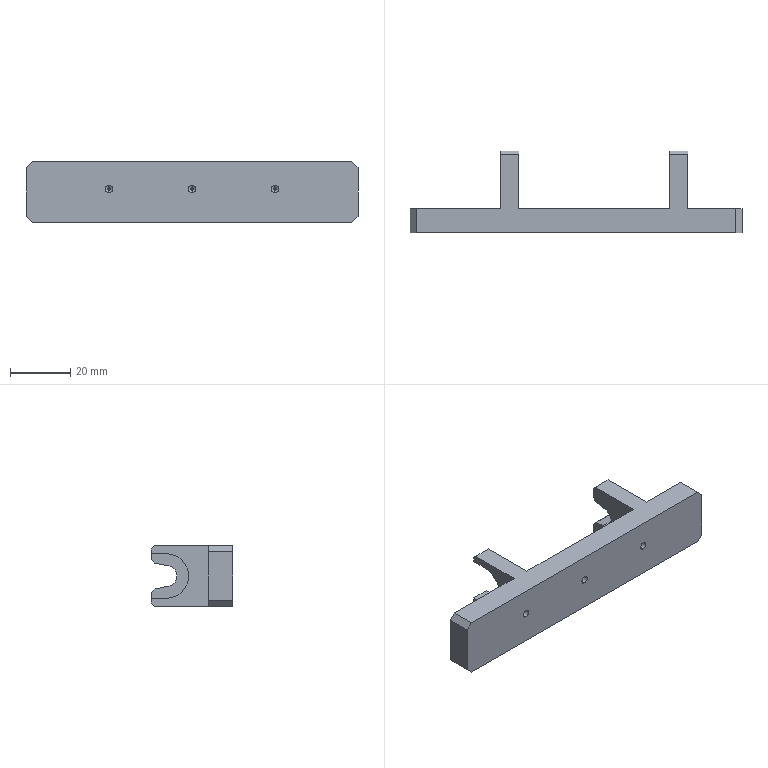Part | STEP file | 012-6-07-03 | 1 solid | 44 faces | box 110 x 27 x 20 mm | volume 20647 mm3 | plane 30 | cylinder 8 | cone 6 | commonest cylinder face diameters 2.5 x6 7 x1 14.8 x1